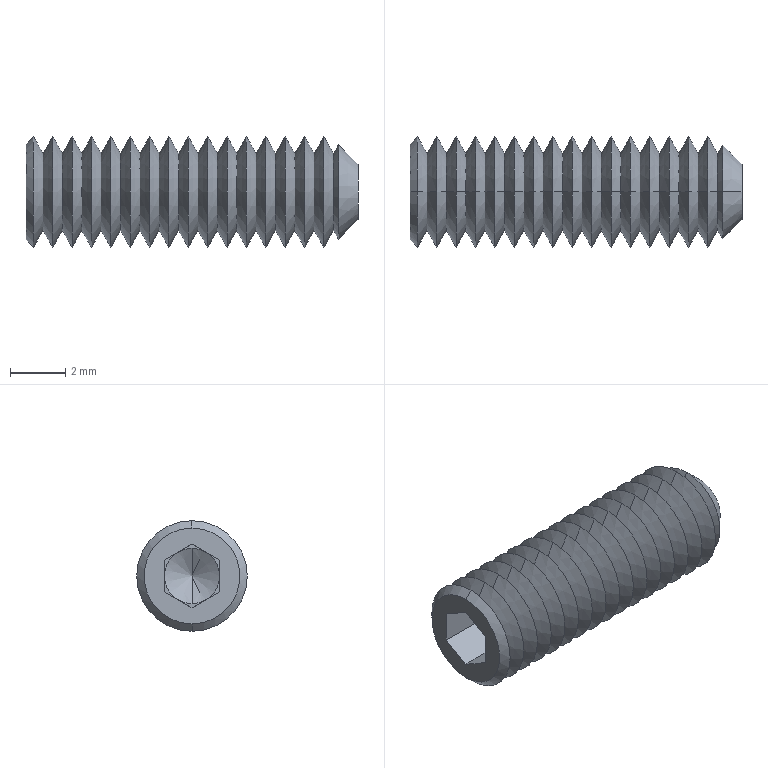Part | STEP file | 1 solid | 85 faces | box 12 x 4 x 4 mm | volume 101.25 mm3 | cone 72 | plane 13